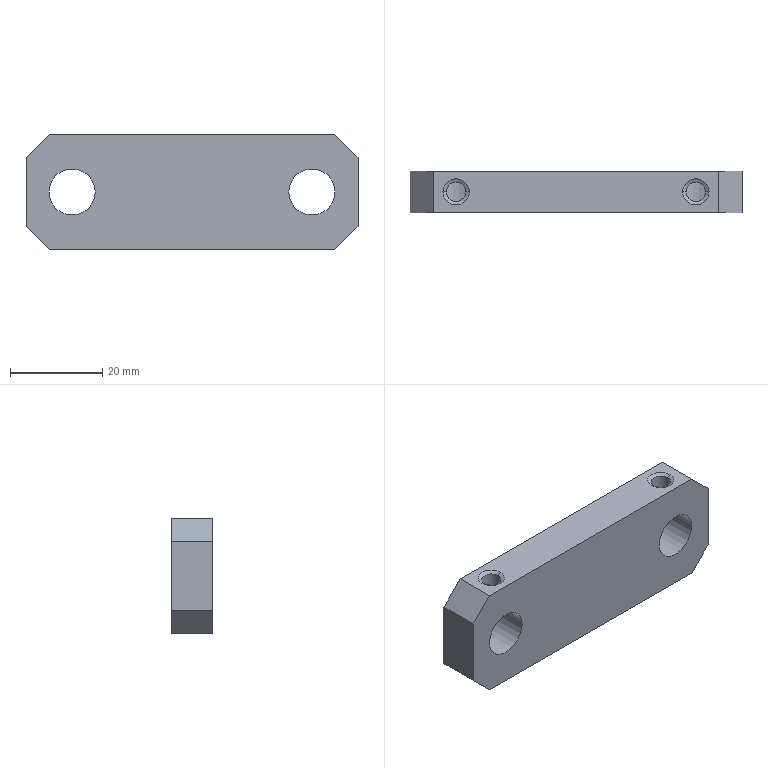Part | NX | 1 solid | 22 faces | box 72 x 9 x 25 mm | volume 14120 mm3 | plane 10 | cylinder 8 | cone 4 | commonest cylinder face diameters 4.2 x4 10 x4
STEP:
#1=CARTESIAN_POINT('',(36.,-4.5,7.5));
#2=VERTEX_POINT('',#1);
#3=CARTESIAN_POINT('',(31.,-4.5,12.5));
#4=VERTEX_POINT('',#3);
#5=CARTESIAN_POINT('',(43.5,-4.5,0.));
#6=DIRECTION('',(-0.7071,0.,0.7071));
#7=VECTOR('',#6,1000.);
#8=LINE('',#5,#7);
#9=EDGE_CURVE('',#2,#4,#8,.T.);
#10=ORIENTED_EDGE('',*,*,#9,.T.);
#11=CARTESIAN_POINT('',(-31.,-4.5,12.5));
#12=VERTEX_POINT('',#11);
#13=CARTESIAN_POINT('',(0.,-4.5,12.5));
#14=DIRECTION('',(-1.,0.,0.));
#15=VECTOR('',#14,1000.);
#16=LINE('',#13,#15);
#17=EDGE_CURVE('',#4,#12,#16,.T.);
#18=ORIENTED_EDGE('',*,*,#17,.T.);
#19=CARTESIAN_POINT('',(-36.,-4.5,7.5));
#20=VERTEX_POINT('',#19);
#21=CARTESIAN_POINT('',(-43.5,-4.5,0.));
#22=DIRECTION('',(-0.7071,0.,-0.7071));
#23=VECTOR('',#22,1000.);
#24=LINE('',#21,#23);
#25=EDGE_CURVE('',#12,#20,#24,.T.);
#26=ORIENTED_EDGE('',*,*,#25,.T.);
#27=CARTESIAN_POINT('',(-36.,-4.5,-7.5));
#28=VERTEX_POINT('',#27);
#29=CARTESIAN_POINT('',(-36.,-4.5,0.));
#30=DIRECTION('',(0.,0.,-1.));
#31=VECTOR('',#30,1000.);
#32=LINE('',#29,#31);
#33=EDGE_CURVE('',#20,#28,#32,.T.);
#34=ORIENTED_EDGE('',*,*,#33,.T.);
#35=CARTESIAN_POINT('',(-31.,-4.5,-12.5));
#36=VERTEX_POINT('',#35);
#37=CARTESIAN_POINT('',(-43.5,-4.5,0.));
#38=DIRECTION('',(0.7071,0.,-0.7071));
#39=VECTOR('',#38,1000.);
#40=LINE('',#37,#39);
#41=EDGE_CURVE('',#28,#36,#40,.T.);
#42=ORIENTED_EDGE('',*,*,#41,.T.);
#43=CARTESIAN_POINT('',(31.,-4.5,-12.5));
#44=VERTEX_POINT('',#43);
#45=CARTESIAN_POINT('',(0.,-4.5,-12.5));
#46=DIRECTION('',(1.,0.,0.));
#47=VECTOR('',#46,1000.);
#48=LINE('',#45,#47);
#49=EDGE_CURVE('',#36,#44,#48,.T.);
#50=ORIENTED_EDGE('',*,*,#49,.T.);
#51=CARTESIAN_POINT('',(36.,-4.5,-7.5));
#52=VERTEX_POINT('',#51);
#53=CARTESIAN_POINT('',(43.5,-4.5,0.));
#54=DIRECTION('',(0.7071,0.,0.7071));
#55=VECTOR('',#54,1000.);
#56=LINE('',#53,#55);
#57=EDGE_CURVE('',#44,#52,#56,.T.);
#58=ORIENTED_EDGE('',*,*,#57,.T.);
#59=CARTESIAN_POINT('',(36.,-4.5,0.));
#60=DIRECTION('',(0.,0.,1.));
#61=VECTOR('',#60,1000.);
#62=LINE('',#59,#61);
#63=EDGE_CURVE('',#52,#2,#62,.T.);
#64=ORIENTED_EDGE('',*,*,#63,.T.);
#65=EDGE_LOOP('',(#10,#18,#26,#34,#42,#50,#58,#64));
#66=FACE_BOUND('',#65,.T.);
#67=CARTESIAN_POINT('',(-31.,-4.5,0.));
#68=VERTEX_POINT('',#67);
#69=CARTESIAN_POINT('',(-21.,-4.5,0.));
#70=VERTEX_POINT('',#69);
#71=CARTESIAN_POINT('',(-26.,-4.5,0.));
#72=DIRECTION('',(0.,-1.,0.));
#73=DIRECTION('',(-1.,0.,0.));
#74=AXIS2_PLACEMENT_3D('',#71,#72,#73);
#75=CIRCLE('',#74,5.);
#76=EDGE_CURVE('',#68,#70,#75,.T.);
#77=ORIENTED_EDGE('',*,*,#76,.F.);
#78=CARTESIAN_POINT('',(-26.,-4.5,0.));
#79=DIRECTION('',(0.,-1.,0.));
#80=DIRECTION('',(-1.,0.,0.));
#81=AXIS2_PLACEMENT_3D('',#78,#79,#80);
#82=CIRCLE('',#81,5.);
#83=EDGE_CURVE('',#70,#68,#82,.T.);
#84=ORIENTED_EDGE('',*,*,#83,.F.);
#85=EDGE_LOOP('',(#77,#84));
#86=FACE_BOUND('',#85,.T.);
#87=CARTESIAN_POINT('',(31.,-4.5,0.));
#88=VERTEX_POINT('',#87);
#89=CARTESIAN_POINT('',(21.,-4.5,0.));
#90=VERTEX_POINT('',#89);
#91=CARTESIAN_POINT('',(26.,-4.5,0.));
#92=DIRECTION('',(0.,-1.,0.));
#93=DIRECTION('',(-1.,0.,0.));
#94=AXIS2_PLACEMENT_3D('',#91,#92,#93);
#95=CIRCLE('',#94,5.);
#96=EDGE_CURVE('',#88,#90,#95,.T.);
#97=ORIENTED_EDGE('',*,*,#96,.F.);
#98=CARTESIAN_POINT('',(26.,-4.5,0.));
#99=DIRECTION('',(0.,-1.,0.));
#100=DIRECTION('',(-1.,0.,0.));
#101=AXIS2_PLACEMENT_3D('',#98,#99,#100);
#102=CIRCLE('',#101,5.);
#103=EDGE_CURVE('',#90,#88,#102,.T.);
#104=ORIENTED_EDGE('',*,*,#103,.F.);
#105=EDGE_LOOP('',(#97,#104));
#106=FACE_BOUND('',#105,.T.);
#107=CARTESIAN_POINT('',(0.,-4.5,0.));
#108=DIRECTION('',(0.,1.,0.));
#109=DIRECTION('',(1.,0.,0.));
#110=AXIS2_PLACEMENT_3D('',#107,#108,#109);
#111=PLANE('',#110);
#112=ADVANCED_FACE('',(#66,#86,#106),#111,.F.);
#113=CARTESIAN_POINT('',(36.,4.5,7.5));
#114=VERTEX_POINT('',#113);
#115=CARTESIAN_POINT('',(36.,-4.5,7.5));
#116=DIRECTION('',(0.,1.,0.));
#117=VECTOR('',#116,1000.);
#118=LINE('',#115,#117);
#119=EDGE_CURVE('',#2,#114,#118,.T.);
#120=ORIENTED_EDGE('',*,*,#119,.F.);
#121=ORIENTED_EDGE('',*,*,#63,.F.);
#122=CARTESIAN_POINT('',(36.,4.5,-7.5));
#123=VERTEX_POINT('',#122);
#124=CARTESIAN_POINT('',(36.,-4.5,-7.5));
#125=DIRECTION('',(0.,1.,0.));
#126=VECTOR('',#125,1000.);
#127=LINE('',#124,#126);
#128=EDGE_CURVE('',#52,#123,#127,.T.);
#129=ORIENTED_EDGE('',*,*,#128,.T.);
#130=CARTESIAN_POINT('',(36.,4.5,0.));
#131=DIRECTION('',(0.,0.,1.));
#132=VECTOR('',#131,1000.);
#133=LINE('',#130,#132);
#134=EDGE_CURVE('',#123,#114,#133,.T.);
#135=ORIENTED_EDGE('',*,*,#134,.T.);
#136=EDGE_LOOP('',(#120,#121,#129,#135));
#137=FACE_BOUND('',#136,.T.);
#138=CARTESIAN_POINT('',(36.,4.5,12.5));
#139=DIRECTION('',(-1.,0.,0.));
#140=DIRECTION('',(0.,0.,1.));
#141=AXIS2_PLACEMENT_3D('',#138,#139,#140);
#142=PLANE('',#141);
#143=ADVANCED_FACE('',(#137),#142,.F.);
#144=CARTESIAN_POINT('',(31.,4.5,12.5));
#145=VERTEX_POINT('',#144);
#146=CARTESIAN_POINT('',(43.5,4.5,0.));
#147=DIRECTION('',(-0.7071,0.,0.7071));
#148=VECTOR('',#147,1000.);
#149=LINE('',#146,#148);
#150=EDGE_CURVE('',#114,#145,#149,.T.);
#151=ORIENTED_EDGE('',*,*,#150,.T.);
#152=CARTESIAN_POINT('',(31.,0.,12.5));
#153=DIRECTION('',(0.,1.,0.));
#154=VECTOR('',#153,1000.);
#155=LINE('',#152,#154);
#156=EDGE_CURVE('',#4,#145,#155,.T.);
#157=ORIENTED_EDGE('',*,*,#156,.F.);
#158=ORIENTED_EDGE('',*,*,#9,.F.);
#159=ORIENTED_EDGE('',*,*,#119,.T.);
#160=EDGE_LOOP('',(#151,#157,#158,#159));
#161=FACE_BOUND('',#160,.T.);
#162=CARTESIAN_POINT('',(36.,4.5,7.5));
#163=DIRECTION('',(-0.7071,0.,-0.7071));
#164=DIRECTION('',(-0.7071,0.,0.7071));
#165=AXIS2_PLACEMENT_3D('',#162,#163,#164);
#166=PLANE('',#165);
#167=ADVANCED_FACE('',(#161),#166,.F.);
#168=CARTESIAN_POINT('',(-31.,4.5,12.5));
#169=VERTEX_POINT('',#168);
#170=CARTESIAN_POINT('',(-31.,0.,12.5));
#171=DIRECTION('',(0.,-1.,0.));
#172=VECTOR('',#171,1000.);
#173=LINE('',#170,#172);
#174=EDGE_CURVE('',#169,#12,#173,.T.);
#175=ORIENTED_EDGE('',*,*,#174,.T.);
#176=ORIENTED_EDGE('',*,*,#17,.F.);
#177=ORIENTED_EDGE('',*,*,#156,.T.);
#178=CARTESIAN_POINT('',(0.,4.5,12.5));
#179=DIRECTION('',(-1.,0.,0.));
#180=VECTOR('',#179,1000.);
#181=LINE('',#178,#180);
#182=EDGE_CURVE('',#145,#169,#181,.T.);
#183=ORIENTED_EDGE('',*,*,#182,.T.);
#184=EDGE_LOOP('',(#175,#176,#177,#183));
#185=FACE_BOUND('',#184,.T.);
#186=CARTESIAN_POINT('',(28.86,0.,12.5));
#187=VERTEX_POINT('',#186);
#188=CARTESIAN_POINT('',(23.14,0.,12.5));
#189=VERTEX_POINT('',#188);
#190=CARTESIAN_POINT('',(26.,0.,12.5));
#191=DIRECTION('',(0.,0.,-1.));
#192=DIRECTION('',(1.,0.,0.));
#193=AXIS2_PLACEMENT_3D('',#190,#191,#192);
#194=CIRCLE('',#193,2.86);
#195=EDGE_CURVE('',#187,#189,#194,.T.);
#196=ORIENTED_EDGE('',*,*,#195,.T.);
#197=CARTESIAN_POINT('',(26.,0.,12.5));
#198=DIRECTION('',(0.,0.,-1.));
#199=DIRECTION('',(1.,0.,0.));
#200=AXIS2_PLACEMENT_3D('',#197,#198,#199);
#201=CIRCLE('',#200,2.86);
#202=EDGE_CURVE('',#189,#187,#201,.T.);
#203=ORIENTED_EDGE('',*,*,#202,.T.);
#204=EDGE_LOOP('',(#196,#203));
#205=FACE_BOUND('',#204,.T.);
#206=CARTESIAN_POINT('',(-23.14,0.,12.5));
#207=VERTEX_POINT('',#206);
#208=CARTESIAN_POINT('',(-28.86,0.,12.5));
#209=VERTEX_POINT('',#208);
#210=CARTESIAN_POINT('',(-26.,0.,12.5));
#211=DIRECTION('',(0.,0.,-1.));
#212=DIRECTION('',(1.,0.,0.));
#213=AXIS2_PLACEMENT_3D('',#210,#211,#212);
#214=CIRCLE('',#213,2.86);
#215=EDGE_CURVE('',#207,#209,#214,.T.);
#216=ORIENTED_EDGE('',*,*,#215,.T.);
#217=CARTESIAN_POINT('',(-26.,0.,12.5));
#218=DIRECTION('',(0.,0.,-1.));
#219=DIRECTION('',(1.,0.,0.));
#220=AXIS2_PLACEMENT_3D('',#217,#218,#219);
#221=CIRCLE('',#220,2.86);
#222=EDGE_CURVE('',#209,#207,#221,.T.);
#223=ORIENTED_EDGE('',*,*,#222,.T.);
#224=EDGE_LOOP('',(#216,#223));
#225=FACE_BOUND('',#224,.T.);
#226=CARTESIAN_POINT('',(-36.,4.5,12.5));
#227=DIRECTION('',(0.,0.,-1.));
#228=DIRECTION('',(0.,-1.,0.));
#229=AXIS2_PLACEMENT_3D('',#226,#227,#228);
#230=PLANE('',#229);
#231=ADVANCED_FACE('',(#185,#205,#225),#230,.F.);
#232=CARTESIAN_POINT('',(-36.,4.5,7.5));
#233=VERTEX_POINT('',#232);
#234=CARTESIAN_POINT('',(-43.5,4.5,0.));
#235=DIRECTION('',(-0.7071,0.,-0.7071));
#236=VECTOR('',#235,1000.);
#237=LINE('',#234,#236);
#238=EDGE_CURVE('',#169,#233,#237,.T.);
#239=ORIENTED_EDGE('',*,*,#238,.T.);
#240=CARTESIAN_POINT('',(-36.,-4.5,7.5));
#241=DIRECTION('',(0.,1.,0.));
#242=VECTOR('',#241,1000.);
#243=LINE('',#240,#242);
#244=EDGE_CURVE('',#20,#233,#243,.T.);
#245=ORIENTED_EDGE('',*,*,#244,.F.);
#246=ORIENTED_EDGE('',*,*,#25,.F.);
#247=ORIENTED_EDGE('',*,*,#174,.F.);
#248=EDGE_LOOP('',(#239,#245,#246,#247));
#249=FACE_BOUND('',#248,.T.);
#250=CARTESIAN_POINT('',(-31.,4.5,12.5));
#251=DIRECTION('',(0.7071,0.,-0.7071));
#252=DIRECTION('',(0.,-1.,0.));
#253=AXIS2_PLACEMENT_3D('',#250,#251,#252);
#254=PLANE('',#253);
#255=ADVANCED_FACE('',(#249),#254,.F.);
#256=CARTESIAN_POINT('',(-36.,4.5,-7.5));
#257=VERTEX_POINT('',#256);
#258=CARTESIAN_POINT('',(-36.,-4.5,-7.5));
#259=DIRECTION('',(0.,1.,0.));
#260=VECTOR('',#259,1000.);
#261=LINE('',#258,#260);
#262=EDGE_CURVE('',#28,#257,#261,.T.);
#263=ORIENTED_EDGE('',*,*,#262,.F.);
#264=ORIENTED_EDGE('',*,*,#33,.F.);
#265=ORIENTED_EDGE('',*,*,#244,.T.);
#266=CARTESIAN_POINT('',(-36.,4.5,0.));
#267=DIRECTION('',(0.,0.,-1.));
#268=VECTOR('',#267,1000.);
#269=LINE('',#266,#268);
#270=EDGE_CURVE('',#233,#257,#269,.T.);
#271=ORIENTED_EDGE('',*,*,#270,.T.);
#272=EDGE_LOOP('',(#263,#264,#265,#271));
#273=FACE_BOUND('',#272,.T.);
#274=CARTESIAN_POINT('',(-36.,4.5,-12.5));
#275=DIRECTION('',(1.,0.,0.));
#276=DIRECTION('',(0.,1.,0.));
#277=AXIS2_PLACEMENT_3D('',#274,#275,#276);
#278=PLANE('',#277);
#279=ADVANCED_FACE('',(#273),#278,.F.);
#280=CARTESIAN_POINT('',(-31.,4.5,-12.5));
#281=VERTEX_POINT('',#280);
#282=CARTESIAN_POINT('',(-43.5,4.5,0.));
#283=DIRECTION('',(0.7071,0.,-0.7071));
#284=VECTOR('',#283,1000.);
#285=LINE('',#282,#284);
#286=EDGE_CURVE('',#257,#281,#285,.T.);
#287=ORIENTED_EDGE('',*,*,#286,.T.);
#288=CARTESIAN_POINT('',(-31.,-4.5,-12.5));
#289=DIRECTION('',(0.,1.,0.));
#290=VECTOR('',#289,1000.);
#291=LINE('',#288,#290);
#292=EDGE_CURVE('',#36,#281,#291,.T.);
#293=ORIENTED_EDGE('',*,*,#292,.F.);
#294=ORIENTED_EDGE('',*,*,#41,.F.);
#295=ORIENTED_EDGE('',*,*,#262,.T.);
#296=EDGE_LOOP('',(#287,#293,#294,#295));
#297=FACE_BOUND('',#296,.T.);
#298=CARTESIAN_POINT('',(-36.,4.5,-7.5));
#299=DIRECTION('',(0.7071,0.,0.7071));
#300=DIRECTION('',(0.,-1.,0.));
#301=AXIS2_PLACEMENT_3D('',#298,#299,#300);
#302=PLANE('',#301);
#303=ADVANCED_FACE('',(#297),#302,.F.);
#304=CARTESIAN_POINT('',(31.,4.5,-12.5));
#305=VERTEX_POINT('',#304);
#306=CARTESIAN_POINT('',(31.,-4.5,-12.5));
#307=DIRECTION('',(0.,1.,0.));
#308=VECTOR('',#307,1000.);
#309=LINE('',#306,#308);
#310=EDGE_CURVE('',#44,#305,#309,.T.);
#311=ORIENTED_EDGE('',*,*,#310,.F.);
#312=ORIENTED_EDGE('',*,*,#49,.F.);
#313=ORIENTED_EDGE('',*,*,#292,.T.);
#314=CARTESIAN_POINT('',(0.,4.5,-12.5));
#315=DIRECTION('',(1.,0.,0.));
#316=VECTOR('',#315,1000.);
#317=LINE('',#314,#316);
#318=EDGE_CURVE('',#281,#305,#317,.T.);
#319=ORIENTED_EDGE('',*,*,#318,.T.);
#320=EDGE_LOOP('',(#311,#312,#313,#319));
#321=FACE_BOUND('',#320,.T.);
#322=CARTESIAN_POINT('',(36.,4.5,-12.5));
#323=DIRECTION('',(0.,0.,1.));
#324=DIRECTION('',(1.,0.,0.));
#325=AXIS2_PLACEMENT_3D('',#322,#323,#324);
#326=PLANE('',#325);
#327=ADVANCED_FACE('',(#321),#326,.F.);
#328=CARTESIAN_POINT('',(43.5,4.5,0.));
#329=DIRECTION('',(0.7071,0.,0.7071));
#330=VECTOR('',#329,1000.);
#331=LINE('',#328,#330);
#332=EDGE_CURVE('',#305,#123,#331,.T.);
#333=ORIENTED_EDGE('',*,*,#332,.T.);
#334=ORIENTED_EDGE('',*,*,#128,.F.);
#335=ORIENTED_EDGE('',*,*,#57,.F.);
#336=ORIENTED_EDGE('',*,*,#310,.T.);
#337=EDGE_LOOP('',(#333,#334,#335,#336));
#338=FACE_BOUND('',#337,.T.);
#339=CARTESIAN_POINT('',(31.,4.5,-12.5));
#340=DIRECTION('',(-0.7071,0.,0.7071));
#341=DIRECTION('',(0.,1.,0.));
#342=AXIS2_PLACEMENT_3D('',#339,#340,#341);
#343=PLANE('',#342);
#344=ADVANCED_FACE('',(#338),#343,.F.);
#345=ORIENTED_EDGE('',*,*,#332,.F.);
#346=ORIENTED_EDGE('',*,*,#318,.F.);
#347=ORIENTED_EDGE('',*,*,#286,.F.);
#348=ORIENTED_EDGE('',*,*,#270,.F.);
#349=ORIENTED_EDGE('',*,*,#238,.F.);
#350=ORIENTED_EDGE('',*,*,#182,.F.);
#351=ORIENTED_EDGE('',*,*,#150,.F.);
#352=ORIENTED_EDGE('',*,*,#134,.F.);
#353=EDGE_LOOP('',(#345,#346,#347,#348,#349,#350,#351,#352));
#354=FACE_BOUND('',#353,.T.);
#355=CARTESIAN_POINT('',(-31.,4.5,0.));
#356=VERTEX_POINT('',#355);
#357=CARTESIAN_POINT('',(-21.,4.5,0.));
#358=VERTEX_POINT('',#357);
#359=CARTESIAN_POINT('',(-26.,4.5,0.));
#360=DIRECTION('',(0.,-1.,0.));
#361=DIRECTION('',(-1.,0.,0.));
#362=AXIS2_PLACEMENT_3D('',#359,#360,#361);
#363=CIRCLE('',#362,5.);
#364=EDGE_CURVE('',#356,#358,#363,.T.);
#365=ORIENTED_EDGE('',*,*,#364,.T.);
#366=CARTESIAN_POINT('',(-26.,4.5,0.));
#367=DIRECTION('',(0.,-1.,0.));
#368=DIRECTION('',(-1.,0.,0.));
#369=AXIS2_PLACEMENT_3D('',#366,#367,#368);
#370=CIRCLE('',#369,5.);
#371=EDGE_CURVE('',#358,#356,#370,.T.);
#372=ORIENTED_EDGE('',*,*,#371,.T.);
#373=EDGE_LOOP('',(#365,#372));
#374=FACE_BOUND('',#373,.T.);
#375=CARTESIAN_POINT('',(21.,4.5,0.));
#376=VERTEX_POINT('',#375);
#377=CARTESIAN_POINT('',(31.,4.5,0.));
#378=VERTEX_POINT('',#377);
#379=CARTESIAN_POINT('',(26.,4.5,0.));
#380=DIRECTION('',(0.,-1.,0.));
#381=DIRECTION('',(-1.,0.,0.));
#382=AXIS2_PLACEMENT_3D('',#379,#380,#381);
#383=CIRCLE('',#382,5.);
#384=EDGE_CURVE('',#376,#378,#383,.T.);
#385=ORIENTED_EDGE('',*,*,#384,.T.);
#386=CARTESIAN_POINT('',(26.,4.5,0.));
#387=DIRECTION('',(0.,-1.,0.));
#388=DIRECTION('',(-1.,0.,0.));
#389=AXIS2_PLACEMENT_3D('',#386,#387,#388);
#390=CIRCLE('',#389,5.);
#391=EDGE_CURVE('',#378,#376,#390,.T.);
#392=ORIENTED_EDGE('',*,*,#391,.T.);
#393=EDGE_LOOP('',(#385,#392));
#394=FACE_BOUND('',#393,.T.);
#395=CARTESIAN_POINT('',(0.,4.5,0.));
#396=DIRECTION('',(0.,1.,0.));
#397=DIRECTION('',(1.,0.,0.));
#398=AXIS2_PLACEMENT_3D('',#395,#396,#397);
#399=PLANE('',#398);
#400=ADVANCED_FACE('',(#354,#374,#394),#399,.T.);
#401=ORIENTED_EDGE('',*,*,#76,.T.);
#402=CARTESIAN_POINT('',(-21.,-4.5,0.));
#403=DIRECTION('',(0.,1.,0.));
#404=VECTOR('',#403,1000.);
#405=LINE('',#402,#404);
#406=EDGE_CURVE('',#358,#70,#405,.F.);
#407=ORIENTED_EDGE('',*,*,#406,.F.);
#408=ORIENTED_EDGE('',*,*,#364,.F.);
#409=CARTESIAN_POINT('',(-31.,-4.5,0.));
#410=DIRECTION('',(0.,1.,0.));
#411=VECTOR('',#410,1000.);
#412=LINE('',#409,#411);
#413=EDGE_CURVE('',#356,#68,#412,.F.);
#414=ORIENTED_EDGE('',*,*,#413,.T.);
#415=EDGE_LOOP('',(#401,#407,#408,#414));
#416=FACE_BOUND('',#415,.T.);
#417=CARTESIAN_POINT('',(-26.,-4.5,0.));
#418=DIRECTION('',(0.,1.,0.));
#419=DIRECTION('',(-1.,0.,0.));
#420=AXIS2_PLACEMENT_3D('',#417,#418,#419);
#421=CYLINDRICAL_SURFACE('',#420,5.);
#422=ADVANCED_FACE('',(#416),#421,.F.);
#423=ORIENTED_EDGE('',*,*,#96,.T.);
#424=CARTESIAN_POINT('',(21.,-4.5,0.));
#425=DIRECTION('',(0.,1.,0.));
#426=VECTOR('',#425,1000.);
#427=LINE('',#424,#426);
#428=EDGE_CURVE('',#376,#90,#427,.F.);
#429=ORIENTED_EDGE('',*,*,#428,.F.);
#430=ORIENTED_EDGE('',*,*,#391,.F.);
#431=CARTESIAN_POINT('',(31.,-4.5,0.));
#432=DIRECTION('',(0.,1.,0.));
#433=VECTOR('',#432,1000.);
#434=LINE('',#431,#433);
#435=EDGE_CURVE('',#378,#88,#434,.F.);
#436=ORIENTED_EDGE('',*,*,#435,.T.);
#437=EDGE_LOOP('',(#423,#429,#430,#436));
#438=FACE_BOUND('',#437,.T.);
#439=CARTESIAN_POINT('',(23.9,0.,4.538));
#440=VERTEX_POINT('',#439);
#441=CARTESIAN_POINT('',(28.1,0.,4.538));
#442=VERTEX_POINT('',#441);
#443=CARTESIAN_POINT('',(23.9,0.,4.538));
#444=CARTESIAN_POINT('',(23.9,-0.556,4.538));
#445=CARTESIAN_POINT('',(24.353,-1.641,4.78));
#446=CARTESIAN_POINT('',(26.,-2.33,5.11));
#447=CARTESIAN_POINT('',(27.646,-1.641,4.78));
#448=CARTESIAN_POINT('',(28.1,-0.556,4.538));
#449=CARTESIAN_POINT('',(28.1,0.,4.538));
#450=B_SPLINE_CURVE_WITH_KNOTS('',3,(#443,#444,#445,#446,#447,#448,#449),.UNSPECIFIED.,.F.,.F.,(4,1,1,1,4),(0.,0.25,0.5,0.75,1.),.UNSPECIFIED.);
#451=EDGE_CURVE('',#440,#442,#450,.T.);
#452=ORIENTED_EDGE('',*,*,#451,.T.);
#453=CARTESIAN_POINT('',(28.1,0.,4.538));
#454=CARTESIAN_POINT('',(28.1,0.5561,4.538));
#455=CARTESIAN_POINT('',(27.647,1.641,4.78));
#456=CARTESIAN_POINT('',(26.,2.329,5.11));
#457=CARTESIAN_POINT('',(24.354,1.642,4.78));
#458=CARTESIAN_POINT('',(23.9,0.5556,4.538));
#459=CARTESIAN_POINT('',(23.9,0.,4.538));
#460=B_SPLINE_CURVE_WITH_KNOTS('',3,(#453,#454,#455,#456,#457,#458,#459),.UNSPECIFIED.,.F.,.F.,(4,1,1,1,4),(0.,0.25,0.5,0.75,1.),.UNSPECIFIED.);
#461=EDGE_CURVE('',#442,#440,#460,.T.);
#462=ORIENTED_EDGE('',*,*,#461,.T.);
#463=EDGE_LOOP('',(#452,#462));
#464=FACE_BOUND('',#463,.T.);
#465=CARTESIAN_POINT('',(26.,-4.5,0.));
#466=DIRECTION('',(0.,1.,0.));
#467=DIRECTION('',(-1.,0.,0.));
#468=AXIS2_PLACEMENT_3D('',#465,#466,#467);
#469=CYLINDRICAL_SURFACE('',#468,5.);
#470=ADVANCED_FACE('',(#438,#464),#469,.F.);
#471=ORIENTED_EDGE('',*,*,#451,.F.);
#472=CARTESIAN_POINT('',(23.9,0.,12.061));
#473=VERTEX_POINT('',#472);
#474=CARTESIAN_POINT('',(23.9,0.,12.5));
#475=DIRECTION('',(0.,0.,1.));
#476=VECTOR('',#475,1000.);
#477=LINE('',#474,#476);
#478=EDGE_CURVE('',#473,#440,#477,.F.);
#479=ORIENTED_EDGE('',*,*,#478,.F.);
#480=CARTESIAN_POINT('',(28.1,0.,12.061));
#481=VERTEX_POINT('',#480);
#482=CARTESIAN_POINT('',(26.,0.,12.061));
#483=DIRECTION('',(0.,0.,-1.));
#484=DIRECTION('',(1.,0.,0.));
#485=AXIS2_PLACEMENT_3D('',#482,#483,#484);
#486=CIRCLE('',#485,2.1);
#487=EDGE_CURVE('',#481,#473,#486,.T.);
#488=ORIENTED_EDGE('',*,*,#487,.F.);
#489=CARTESIAN_POINT('',(28.1,0.,12.5));
#490=DIRECTION('',(0.,0.,1.));
#491=VECTOR('',#490,1000.);
#492=LINE('',#489,#491);
#493=EDGE_CURVE('',#481,#442,#492,.F.);
#494=ORIENTED_EDGE('',*,*,#493,.T.);
#495=EDGE_LOOP('',(#471,#479,#488,#494));
#496=FACE_BOUND('',#495,.T.);
#497=CARTESIAN_POINT('',(26.,0.,12.5));
#498=DIRECTION('',(0.,0.,1.));
#499=DIRECTION('',(1.,0.,0.));
#500=AXIS2_PLACEMENT_3D('',#497,#498,#499);
#501=CYLINDRICAL_SURFACE('',#500,2.1);
#502=ADVANCED_FACE('',(#496),#501,.F.);
#503=CARTESIAN_POINT('',(26.,0.,12.061));
#504=DIRECTION('',(0.,0.,-1.));
#505=DIRECTION('',(1.,0.,0.));
#506=AXIS2_PLACEMENT_3D('',#503,#504,#505);
#507=CIRCLE('',#506,2.1);
#508=EDGE_CURVE('',#473,#481,#507,.T.);
#509=ORIENTED_EDGE('',*,*,#508,.T.);
#510=CARTESIAN_POINT('',(28.1,0.,12.061));
#511=DIRECTION('',(0.866,0.,0.5));
#512=VECTOR('',#511,1000.);
#513=LINE('',#510,#512);
#514=EDGE_CURVE('',#481,#187,#513,.T.);
#515=ORIENTED_EDGE('',*,*,#514,.T.);
#516=ORIENTED_EDGE('',*,*,#202,.F.);
#517=CARTESIAN_POINT('',(23.9,0.,12.061));
#518=DIRECTION('',(-0.866,0.,0.5));
#519=VECTOR('',#518,1000.);
#520=LINE('',#517,#519);
#521=EDGE_CURVE('',#473,#189,#520,.T.);
#522=ORIENTED_EDGE('',*,*,#521,.F.);
#523=EDGE_LOOP('',(#509,#515,#516,#522));
#524=FACE_BOUND('',#523,.T.);
#525=CARTESIAN_POINT('',(26.,0.,12.061));
#526=DIRECTION('',(0.,0.,1.));
#527=DIRECTION('',(1.,0.,0.));
#528=AXIS2_PLACEMENT_3D('',#525,#526,#527);
#529=CONICAL_SURFACE('',#528,2.1,1.047);
#530=ADVANCED_FACE('',(#524),#529,.F.);
#531=CARTESIAN_POINT('',(-23.9,0.,4.538));
#532=VERTEX_POINT('',#531);
#533=CARTESIAN_POINT('',(-28.1,0.,4.538));
#534=VERTEX_POINT('',#533);
#535=CARTESIAN_POINT('',(-23.9,0.,4.538));
#536=CARTESIAN_POINT('',(-23.9,-0.1282,4.538));
#537=CARTESIAN_POINT('',(-23.917,-0.3832,4.547));
#538=CARTESIAN_POINT('',(-24.07,-0.8514,4.612));
#539=CARTESIAN_POINT('',(-24.177,-1.065,4.659));
#540=CARTESIAN_POINT('',(-24.503,-1.51,4.777));
#541=CARTESIAN_POINT('',(-24.899,-1.799,4.879));
#542=CARTESIAN_POINT('',(-25.161,-1.938,4.933));
#543=CARTESIAN_POINT('',(-25.612,-2.081,4.991));
#544=CARTESIAN_POINT('',(-26.,-2.109,5.005));
#545=CARTESIAN_POINT('',(-26.387,-2.081,4.991));
#546=CARTESIAN_POINT('',(-26.839,-1.938,4.933));
#547=CARTESIAN_POINT('',(-27.101,-1.799,4.879));
#548=CARTESIAN_POINT('',(-27.497,-1.511,4.777));
#549=CARTESIAN_POINT('',(-27.823,-1.066,4.659));
#550=CARTESIAN_POINT('',(-27.93,-0.8513,4.612));
#551=CARTESIAN_POINT('',(-28.083,-0.3833,4.547));
#552=CARTESIAN_POINT('',(-28.1,-0.1282,4.538));
#553=CARTESIAN_POINT('',(-28.1,0.,4.538));
#554=B_SPLINE_CURVE_WITH_KNOTS('',3,(#535,#536,#537,#538,#539,#540,#541,#542,#543,#544,#545,#546,#547,#548,#549,#550,#551,#552,#553),.UNSPECIFIED.,.F.,.F.,(4,1,1,1,1,1,1,1,1,1,1,1,1,1,1,1,4),(0.,0.0625,0.125,0.1875,0.25,0.3125,0.375,0.4375,0.5,0.5625,0.625,0.6875,0.75,0.8125,0.875,0.9375,1.),.UNSPECIFIED.);
#555=EDGE_CURVE('',#532,#534,#554,.T.);
#556=ORIENTED_EDGE('',*,*,#555,.T.);
#557=CARTESIAN_POINT('',(-28.1,0.,12.061));
#558=VERTEX_POINT('',#557);
#559=CARTESIAN_POINT('',(-28.1,0.,12.5));
#560=DIRECTION('',(0.,0.,1.));
#561=VECTOR('',#560,1000.);
#562=LINE('',#559,#561);
#563=EDGE_CURVE('',#534,#558,#562,.T.);
#564=ORIENTED_EDGE('',*,*,#563,.T.);
#565=CARTESIAN_POINT('',(-23.9,0.,12.061));
#566=VERTEX_POINT('',#565);
#567=CARTESIAN_POINT('',(-26.,0.,12.061));
#568=DIRECTION('',(0.,0.,-1.));
#569=DIRECTION('',(1.,0.,0.));
#570=AXIS2_PLACEMENT_3D('',#567,#568,#569);
#571=CIRCLE('',#570,2.1);
#572=EDGE_CURVE('',#566,#558,#571,.T.);
#573=ORIENTED_EDGE('',*,*,#572,.F.);
#574=CARTESIAN_POINT('',(-23.9,0.,12.5));
#575=DIRECTION('',(0.,0.,1.));
#576=VECTOR('',#575,1000.);
#577=LINE('',#574,#576);
#578=EDGE_CURVE('',#532,#566,#577,.T.);
#579=ORIENTED_EDGE('',*,*,#578,.F.);
#580=EDGE_LOOP('',(#556,#564,#573,#579));
#581=FACE_BOUND('',#580,.T.);
#582=CARTESIAN_POINT('',(-26.,0.,12.5));
#583=DIRECTION('',(0.,0.,1.));
#584=DIRECTION('',(1.,0.,0.));
#585=AXIS2_PLACEMENT_3D('',#582,#583,#584);
#586=CYLINDRICAL_SURFACE('',#585,2.1);
#587=ADVANCED_FACE('',(#581),#586,.F.);
#588=ORIENTED_EDGE('',*,*,#215,.F.);
#589=CARTESIAN_POINT('',(-23.9,0.,12.061));
#590=DIRECTION('',(0.866,0.,0.5));
#591=VECTOR('',#590,1000.);
#592=LINE('',#589,#591);
#593=EDGE_CURVE('',#566,#207,#592,.T.);
#594=ORIENTED_EDGE('',*,*,#593,.F.);
#595=ORIENTED_EDGE('',*,*,#572,.T.);
#596=CARTESIAN_POINT('',(-28.1,0.,12.061));
#597=DIRECTION('',(-0.866,0.,0.5));
#598=VECTOR('',#597,1000.);
#599=LINE('',#596,#598);
#600=EDGE_CURVE('',#558,#209,#599,.T.);
#601=ORIENTED_EDGE('',*,*,#600,.T.);
#602=EDGE_LOOP('',(#588,#594,#595,#601));
#603=FACE_BOUND('',#602,.T.);
#604=CARTESIAN_POINT('',(-26.,0.,12.061));
#605=DIRECTION('',(0.,0.,1.));
#606=DIRECTION('',(1.,0.,0.));
#607=AXIS2_PLACEMENT_3D('',#604,#605,#606);
#608=CONICAL_SURFACE('',#607,2.1,1.047);
#609=ADVANCED_FACE('',(#603),#608,.F.);
#610=ORIENTED_EDGE('',*,*,#195,.F.);
#611=ORIENTED_EDGE('',*,*,#514,.F.);
#612=ORIENTED_EDGE('',*,*,#487,.T.);
#613=ORIENTED_EDGE('',*,*,#521,.T.);
#614=EDGE_LOOP('',(#610,#611,#612,#613));
#615=FACE_BOUND('',#614,.T.);
#616=CARTESIAN_POINT('',(26.,0.,12.061));
#617=DIRECTION('',(0.,0.,1.));
#618=DIRECTION('',(1.,0.,0.));
#619=AXIS2_PLACEMENT_3D('',#616,#617,#618);
#620=CONICAL_SURFACE('',#619,2.1,1.047);
#621=ADVANCED_FACE('',(#615),#620,.F.);
#622=ORIENTED_EDGE('',*,*,#593,.T.);
#623=ORIENTED_EDGE('',*,*,#222,.F.);
#624=ORIENTED_EDGE('',*,*,#600,.F.);
#625=CARTESIAN_POINT('',(-26.,0.,12.061));
#626=DIRECTION('',(0.,0.,-1.));
#627=DIRECTION('',(1.,0.,0.));
#628=AXIS2_PLACEMENT_3D('',#625,#626,#627);
#629=CIRCLE('',#628,2.1);
#630=EDGE_CURVE('',#558,#566,#629,.T.);
#631=ORIENTED_EDGE('',*,*,#630,.T.);
#632=EDGE_LOOP('',(#622,#623,#624,#631));
#633=FACE_BOUND('',#632,.T.);
#634=CARTESIAN_POINT('',(-26.,0.,12.061));
#635=DIRECTION('',(0.,0.,1.));
#636=DIRECTION('',(1.,0.,0.));
#637=AXIS2_PLACEMENT_3D('',#634,#635,#636);
#638=CONICAL_SURFACE('',#637,2.1,1.047);
#639=ADVANCED_FACE('',(#633),#638,.F.);
#640=ORIENTED_EDGE('',*,*,#578,.T.);
#641=ORIENTED_EDGE('',*,*,#630,.F.);
#642=ORIENTED_EDGE('',*,*,#563,.F.);
#643=CARTESIAN_POINT('',(-28.1,0.,4.538));
#644=CARTESIAN_POINT('',(-28.1,0.1282,4.538));
#645=CARTESIAN_POINT('',(-28.083,0.3833,4.547));
#646=CARTESIAN_POINT('',(-27.93,0.8513,4.612));
#647=CARTESIAN_POINT('',(-27.823,1.065,4.659));
#648=CARTESIAN_POINT('',(-27.497,1.51,4.777));
#649=CARTESIAN_POINT('',(-27.101,1.799,4.879));
#650=CARTESIAN_POINT('',(-26.839,1.938,4.933));
#651=CARTESIAN_POINT('',(-26.388,2.081,4.991));
#652=CARTESIAN_POINT('',(-26.,2.109,5.005));
#653=CARTESIAN_POINT('',(-25.613,2.081,4.991));
#654=CARTESIAN_POINT('',(-25.161,1.938,4.933));
#655=CARTESIAN_POINT('',(-24.899,1.799,4.879));
#656=CARTESIAN_POINT('',(-24.503,1.511,4.777));
#657=CARTESIAN_POINT('',(-24.177,1.065,4.659));
#658=CARTESIAN_POINT('',(-24.07,0.8513,4.612));
#659=CARTESIAN_POINT('',(-23.917,0.383,4.547));
#660=CARTESIAN_POINT('',(-23.9,0.1281,4.538));
#661=CARTESIAN_POINT('',(-23.9,0.,4.538));
#662=B_SPLINE_CURVE_WITH_KNOTS('',3,(#643,#644,#645,#646,#647,#648,#649,#650,#651,#652,#653,#654,#655,#656,#657,#658,#659,#660,#661),.UNSPECIFIED.,.F.,.F.,(4,1,1,1,1,1,1,1,1,1,1,1,1,1,1,1,4),(0.,0.0625,0.125,0.1875,0.25,0.3125,0.375,0.4375,0.5,0.5625,0.625,0.6875,0.75,0.8125,0.875,0.9375,1.),.UNSPECIFIED.);
#663=EDGE_CURVE('',#534,#532,#662,.T.);
#664=ORIENTED_EDGE('',*,*,#663,.T.);
#665=EDGE_LOOP('',(#640,#641,#642,#664));
#666=FACE_BOUND('',#665,.T.);
#667=CARTESIAN_POINT('',(-26.,0.,12.5));
#668=DIRECTION('',(0.,0.,1.));
#669=DIRECTION('',(1.,0.,0.));
#670=AXIS2_PLACEMENT_3D('',#667,#668,#669);
#671=CYLINDRICAL_SURFACE('',#670,2.1);
#672=ADVANCED_FACE('',(#666),#671,.F.);
#673=ORIENTED_EDGE('',*,*,#413,.F.);
#674=ORIENTED_EDGE('',*,*,#371,.F.);
#675=ORIENTED_EDGE('',*,*,#406,.T.);
#676=ORIENTED_EDGE('',*,*,#83,.T.);
#677=EDGE_LOOP('',(#673,#674,#675,#676));
#678=FACE_BOUND('',#677,.T.);
#679=ORIENTED_EDGE('',*,*,#663,.F.);
#680=ORIENTED_EDGE('',*,*,#555,.F.);
#681=EDGE_LOOP('',(#679,#680));
#682=FACE_BOUND('',#681,.T.);
#683=CARTESIAN_POINT('',(-26.,-4.5,0.));
#684=DIRECTION('',(0.,1.,0.));
#685=DIRECTION('',(-1.,0.,0.));
#686=AXIS2_PLACEMENT_3D('',#683,#684,#685);
#687=CYLINDRICAL_SURFACE('',#686,5.);
#688=ADVANCED_FACE('',(#678,#682),#687,.F.);
#689=ORIENTED_EDGE('',*,*,#384,.F.);
#690=ORIENTED_EDGE('',*,*,#428,.T.);
#691=ORIENTED_EDGE('',*,*,#103,.T.);
#692=ORIENTED_EDGE('',*,*,#435,.F.);
#693=EDGE_LOOP('',(#689,#690,#691,#692));
#694=FACE_BOUND('',#693,.T.);
#695=CARTESIAN_POINT('',(26.,-4.5,0.));
#696=DIRECTION('',(0.,1.,0.));
#697=DIRECTION('',(-1.,0.,0.));
#698=AXIS2_PLACEMENT_3D('',#695,#696,#697);
#699=CYLINDRICAL_SURFACE('',#698,5.);
#700=ADVANCED_FACE('',(#694),#699,.F.);
#701=ORIENTED_EDGE('',*,*,#508,.F.);
#702=ORIENTED_EDGE('',*,*,#478,.T.);
#703=ORIENTED_EDGE('',*,*,#461,.F.);
#704=ORIENTED_EDGE('',*,*,#493,.F.);
#705=EDGE_LOOP('',(#701,#702,#703,#704));
#706=FACE_BOUND('',#705,.T.);
#707=CARTESIAN_POINT('',(26.,0.,12.5));
#708=DIRECTION('',(0.,0.,1.));
#709=DIRECTION('',(1.,0.,0.));
#710=AXIS2_PLACEMENT_3D('',#707,#708,#709);
#711=CYLINDRICAL_SURFACE('',#710,2.1);
#712=ADVANCED_FACE('',(#706),#711,.F.);
#713=CLOSED_SHELL('',(#112,#143,#167,#231,#255,#279,#303,#327,#344,#400,#422,#470,#502,#530,#587,#609,#621,#639,#672,#688,#700,#712));
#714=MANIFOLD_SOLID_BREP('',#713);
#715=(LENGTH_UNIT()NAMED_UNIT(*)SI_UNIT(.MILLI.,.METRE.));
#716=UNCERTAINTY_MEASURE_WITH_UNIT(LENGTH_MEASURE(0.0508),#715,'','');
#717=(NAMED_UNIT(*)PLANE_ANGLE_UNIT()SI_UNIT($,.RADIAN.));
#718=(NAMED_UNIT(*)SI_UNIT($,.STERADIAN.)SOLID_ANGLE_UNIT());
#719=(GEOMETRIC_REPRESENTATION_CONTEXT(3)GLOBAL_UNCERTAINTY_ASSIGNED_CONTEXT((#716))GLOBAL_UNIT_ASSIGNED_CONTEXT((#715,#717,#718))REPRESENTATION_CONTEXT('',''));
#720=ADVANCED_BREP_SHAPE_REPRESENTATION('',(#714),#719);